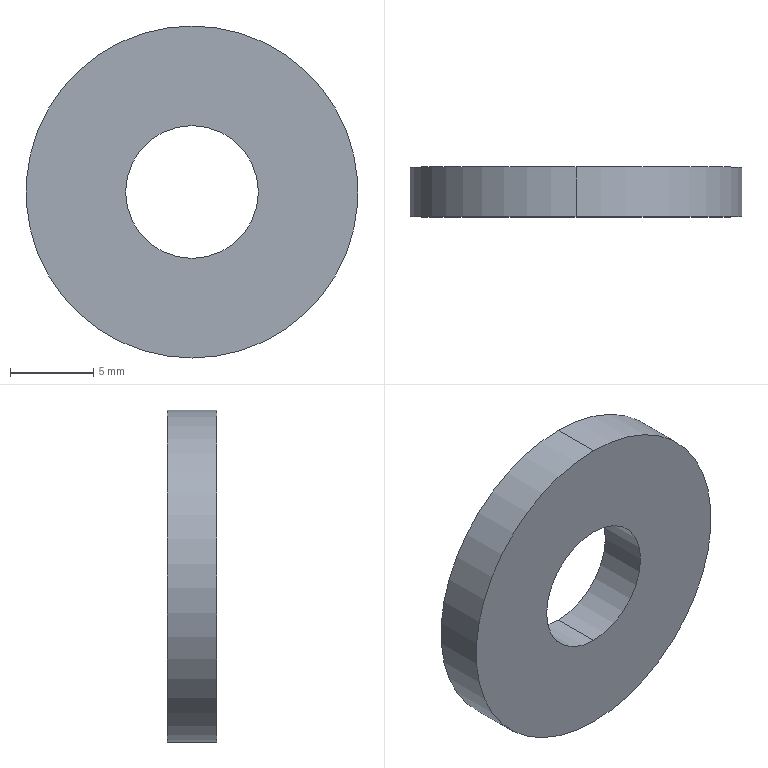Part | STEP file | Cuon T phu H01_8 | 1 solid | 6 faces | box 20 x 3 x 20 mm | volume 791.681 mm3 | cylinder 4 | plane 2 | commonest cylinder face diameters 8 x2 20 x2
STEP:
#1=CARTESIAN_POINT('',(0.,0.,0.));
#2=DIRECTION('',(0.,0.,1.));
#3=DIRECTION('',(1.,0.,0.));
#4=AXIS2_PLACEMENT_3D('',#1,#2,#3);
#5=CARTESIAN_POINT('',(0.,3.,-4.));
#6=VERTEX_POINT('',#5);
#7=CARTESIAN_POINT('',(0.,0.,-4.));
#8=VERTEX_POINT('',#7);
#9=CARTESIAN_POINT('',(0.,3.,-4.));
#10=DIRECTION('',(0.,-1.,0.));
#11=VECTOR('',#10,1.);
#12=LINE('',#9,#11);
#13=CARTESIAN_POINT('',(0.,3.,0.));
#14=DIRECTION('',(0.,-1.,0.));
#15=DIRECTION('',(0.,0.,-1.));
#16=AXIS2_PLACEMENT_3D('',#13,#14,#15);
#17=CYLINDRICAL_SURFACE('',#16,4.);
#18=CARTESIAN_POINT('',(6.283,0.));
#19=DIRECTION('',(0.,1.));
#20=VECTOR('',#19,1.);
#21=LINE('',#18,#20);
#22=(GEOMETRIC_REPRESENTATION_CONTEXT(2)PARAMETRIC_REPRESENTATION_CONTEXT()REPRESENTATION_CONTEXT('',''));
#23=DEFINITIONAL_REPRESENTATION('',(#21),#22);
#24=PCURVE('',#17,#23);
#25=CARTESIAN_POINT('',(0.,3.,0.));
#26=DIRECTION('',(0.,-1.,0.));
#27=DIRECTION('',(0.,0.,-1.));
#28=AXIS2_PLACEMENT_3D('',#25,#26,#27);
#29=CYLINDRICAL_SURFACE('',#28,4.);
#30=CARTESIAN_POINT('',(0.,0.));
#31=DIRECTION('',(0.,1.));
#32=VECTOR('',#31,1.);
#33=LINE('',#30,#32);
#34=(GEOMETRIC_REPRESENTATION_CONTEXT(2)PARAMETRIC_REPRESENTATION_CONTEXT()REPRESENTATION_CONTEXT('',''));
#35=DEFINITIONAL_REPRESENTATION('',(#33),#34);
#36=PCURVE('',#29,#35);
#37=SURFACE_CURVE('',#12,(#24,#36),.PCURVE_S1.);
#38=EDGE_CURVE('',#6,#8,#37,.T.);
#39=ORIENTED_EDGE('',*,*,#38,.T.);
#40=CARTESIAN_POINT('',(0.,0.,4.));
#41=VERTEX_POINT('',#40);
#42=CARTESIAN_POINT('',(0.,0.,0.));
#43=DIRECTION('',(0.,1.,0.));
#44=DIRECTION('',(0.,0.,1.));
#45=AXIS2_PLACEMENT_3D('',#42,#43,#44);
#46=CIRCLE('',#45,4.);
#47=CARTESIAN_POINT('',(9.425,3.));
#48=DIRECTION('',(-1.,0.));
#49=VECTOR('',#48,1.);
#50=LINE('',#47,#49);
#51=(GEOMETRIC_REPRESENTATION_CONTEXT(2)PARAMETRIC_REPRESENTATION_CONTEXT()REPRESENTATION_CONTEXT('',''));
#52=DEFINITIONAL_REPRESENTATION('',(#50),#51);
#53=PCURVE('',#17,#52);
#54=CARTESIAN_POINT('',(0.,0.,0.));
#55=DIRECTION('',(0.,1.,0.));
#56=DIRECTION('',(0.,0.,1.));
#57=AXIS2_PLACEMENT_3D('',#54,#55,#56);
#58=PLANE('',#57);
#59=CARTESIAN_POINT('',(0.,0.));
#60=DIRECTION('',(1.,0.));
#61=AXIS2_PLACEMENT_2D('',#59,#60);
#62=CIRCLE('',#61,4.);
#63=(GEOMETRIC_REPRESENTATION_CONTEXT(2)PARAMETRIC_REPRESENTATION_CONTEXT()REPRESENTATION_CONTEXT('',''));
#64=DEFINITIONAL_REPRESENTATION('',(#62),#63);
#65=PCURVE('',#58,#64);
#66=SURFACE_CURVE('',#46,(#53,#65),.PCURVE_S1.);
#67=EDGE_CURVE('',#8,#41,#66,.T.);
#68=ORIENTED_EDGE('',*,*,#67,.T.);
#69=CARTESIAN_POINT('',(0.,3.,4.));
#70=VERTEX_POINT('',#69);
#71=CARTESIAN_POINT('',(0.,3.,4.));
#72=DIRECTION('',(0.,-1.,0.));
#73=VECTOR('',#72,1.);
#74=LINE('',#71,#73);
#75=CARTESIAN_POINT('',(3.142,0.));
#76=DIRECTION('',(0.,1.));
#77=VECTOR('',#76,1.);
#78=LINE('',#75,#77);
#79=(GEOMETRIC_REPRESENTATION_CONTEXT(2)PARAMETRIC_REPRESENTATION_CONTEXT()REPRESENTATION_CONTEXT('',''));
#80=DEFINITIONAL_REPRESENTATION('',(#78),#79);
#81=PCURVE('',#17,#80);
#82=CARTESIAN_POINT('',(3.142,0.));
#83=DIRECTION('',(0.,1.));
#84=VECTOR('',#83,1.);
#85=LINE('',#82,#84);
#86=(GEOMETRIC_REPRESENTATION_CONTEXT(2)PARAMETRIC_REPRESENTATION_CONTEXT()REPRESENTATION_CONTEXT('',''));
#87=DEFINITIONAL_REPRESENTATION('',(#85),#86);
#88=PCURVE('',#29,#87);
#89=SURFACE_CURVE('',#74,(#81,#88),.PCURVE_S1.);
#90=EDGE_CURVE('',#70,#41,#89,.T.);
#91=ORIENTED_EDGE('',*,*,#90,.F.);
#92=CARTESIAN_POINT('',(0.,3.,0.));
#93=DIRECTION('',(0.,1.,0.));
#94=DIRECTION('',(0.,0.,1.));
#95=AXIS2_PLACEMENT_3D('',#92,#93,#94);
#96=CIRCLE('',#95,4.);
#97=CARTESIAN_POINT('',(9.425,0.));
#98=DIRECTION('',(-1.,0.));
#99=VECTOR('',#98,1.);
#100=LINE('',#97,#99);
#101=(GEOMETRIC_REPRESENTATION_CONTEXT(2)PARAMETRIC_REPRESENTATION_CONTEXT()REPRESENTATION_CONTEXT('',''));
#102=DEFINITIONAL_REPRESENTATION('',(#100),#101);
#103=PCURVE('',#17,#102);
#104=CARTESIAN_POINT('',(0.,3.,0.));
#105=DIRECTION('',(0.,1.,0.));
#106=DIRECTION('',(0.,0.,1.));
#107=AXIS2_PLACEMENT_3D('',#104,#105,#106);
#108=PLANE('',#107);
#109=CARTESIAN_POINT('',(0.,0.));
#110=DIRECTION('',(1.,0.));
#111=AXIS2_PLACEMENT_2D('',#109,#110);
#112=CIRCLE('',#111,4.);
#113=(GEOMETRIC_REPRESENTATION_CONTEXT(2)PARAMETRIC_REPRESENTATION_CONTEXT()REPRESENTATION_CONTEXT('',''));
#114=DEFINITIONAL_REPRESENTATION('',(#112),#113);
#115=PCURVE('',#108,#114);
#116=SURFACE_CURVE('',#96,(#103,#115),.PCURVE_S1.);
#117=EDGE_CURVE('',#6,#70,#116,.T.);
#118=ORIENTED_EDGE('',*,*,#117,.F.);
#119=EDGE_LOOP('',(#39,#68,#91,#118));
#120=FACE_BOUND('',#119,.F.);
#121=ADVANCED_FACE('',(#120),#17,.F.);
#122=CARTESIAN_POINT('',(0.,3.,10.));
#123=VERTEX_POINT('',#122);
#124=CARTESIAN_POINT('',(0.,3.,-10.));
#125=VERTEX_POINT('',#124);
#126=CARTESIAN_POINT('',(0.,3.,0.));
#127=DIRECTION('',(0.,1.,0.));
#128=DIRECTION('',(0.,0.,1.));
#129=AXIS2_PLACEMENT_3D('',#126,#127,#128);
#130=CIRCLE('',#129,10.);
#131=CARTESIAN_POINT('',(0.,3.,0.));
#132=DIRECTION('',(0.,-1.,0.));
#133=DIRECTION('',(0.,0.,-1.));
#134=AXIS2_PLACEMENT_3D('',#131,#132,#133);
#135=CYLINDRICAL_SURFACE('',#134,10.);
#136=CARTESIAN_POINT('',(3.142,0.));
#137=DIRECTION('',(-1.,0.));
#138=VECTOR('',#137,1.);
#139=LINE('',#136,#138);
#140=(GEOMETRIC_REPRESENTATION_CONTEXT(2)PARAMETRIC_REPRESENTATION_CONTEXT()REPRESENTATION_CONTEXT('',''));
#141=DEFINITIONAL_REPRESENTATION('',(#139),#140);
#142=PCURVE('',#135,#141);
#143=CARTESIAN_POINT('',(0.,0.));
#144=DIRECTION('',(1.,0.));
#145=AXIS2_PLACEMENT_2D('',#143,#144);
#146=CIRCLE('',#145,10.);
#147=(GEOMETRIC_REPRESENTATION_CONTEXT(2)PARAMETRIC_REPRESENTATION_CONTEXT()REPRESENTATION_CONTEXT('',''));
#148=DEFINITIONAL_REPRESENTATION('',(#146),#147);
#149=PCURVE('',#108,#148);
#150=SURFACE_CURVE('',#130,(#142,#149),.PCURVE_S1.);
#151=EDGE_CURVE('',#123,#125,#150,.T.);
#152=ORIENTED_EDGE('',*,*,#151,.F.);
#153=CARTESIAN_POINT('',(0.,0.,10.));
#154=VERTEX_POINT('',#153);
#155=CARTESIAN_POINT('',(0.,3.,10.));
#156=DIRECTION('',(0.,-1.,0.));
#157=VECTOR('',#156,1.);
#158=LINE('',#155,#157);
#159=CARTESIAN_POINT('',(3.142,0.));
#160=DIRECTION('',(0.,1.));
#161=VECTOR('',#160,1.);
#162=LINE('',#159,#161);
#163=(GEOMETRIC_REPRESENTATION_CONTEXT(2)PARAMETRIC_REPRESENTATION_CONTEXT()REPRESENTATION_CONTEXT('',''));
#164=DEFINITIONAL_REPRESENTATION('',(#162),#163);
#165=PCURVE('',#135,#164);
#166=CARTESIAN_POINT('',(0.,3.,0.));
#167=DIRECTION('',(0.,-1.,0.));
#168=DIRECTION('',(0.,0.,-1.));
#169=AXIS2_PLACEMENT_3D('',#166,#167,#168);
#170=CYLINDRICAL_SURFACE('',#169,10.);
#171=CARTESIAN_POINT('',(3.142,0.));
#172=DIRECTION('',(0.,1.));
#173=VECTOR('',#172,1.);
#174=LINE('',#171,#173);
#175=(GEOMETRIC_REPRESENTATION_CONTEXT(2)PARAMETRIC_REPRESENTATION_CONTEXT()REPRESENTATION_CONTEXT('',''));
#176=DEFINITIONAL_REPRESENTATION('',(#174),#175);
#177=PCURVE('',#170,#176);
#178=SURFACE_CURVE('',#158,(#165,#177),.PCURVE_S1.);
#179=EDGE_CURVE('',#123,#154,#178,.T.);
#180=ORIENTED_EDGE('',*,*,#179,.T.);
#181=CARTESIAN_POINT('',(0.,0.,-10.));
#182=VERTEX_POINT('',#181);
#183=CARTESIAN_POINT('',(0.,0.,0.));
#184=DIRECTION('',(0.,1.,0.));
#185=DIRECTION('',(0.,0.,1.));
#186=AXIS2_PLACEMENT_3D('',#183,#184,#185);
#187=CIRCLE('',#186,10.);
#188=CARTESIAN_POINT('',(3.142,3.));
#189=DIRECTION('',(-1.,0.));
#190=VECTOR('',#189,1.);
#191=LINE('',#188,#190);
#192=(GEOMETRIC_REPRESENTATION_CONTEXT(2)PARAMETRIC_REPRESENTATION_CONTEXT()REPRESENTATION_CONTEXT('',''));
#193=DEFINITIONAL_REPRESENTATION('',(#191),#192);
#194=PCURVE('',#135,#193);
#195=CARTESIAN_POINT('',(0.,0.));
#196=DIRECTION('',(1.,0.));
#197=AXIS2_PLACEMENT_2D('',#195,#196);
#198=CIRCLE('',#197,10.);
#199=(GEOMETRIC_REPRESENTATION_CONTEXT(2)PARAMETRIC_REPRESENTATION_CONTEXT()REPRESENTATION_CONTEXT('',''));
#200=DEFINITIONAL_REPRESENTATION('',(#198),#199);
#201=PCURVE('',#58,#200);
#202=SURFACE_CURVE('',#187,(#194,#201),.PCURVE_S1.);
#203=EDGE_CURVE('',#154,#182,#202,.T.);
#204=ORIENTED_EDGE('',*,*,#203,.T.);
#205=CARTESIAN_POINT('',(0.,3.,-10.));
#206=DIRECTION('',(0.,-1.,0.));
#207=VECTOR('',#206,1.);
#208=LINE('',#205,#207);
#209=CARTESIAN_POINT('',(0.,0.));
#210=DIRECTION('',(0.,1.));
#211=VECTOR('',#210,1.);
#212=LINE('',#209,#211);
#213=(GEOMETRIC_REPRESENTATION_CONTEXT(2)PARAMETRIC_REPRESENTATION_CONTEXT()REPRESENTATION_CONTEXT('',''));
#214=DEFINITIONAL_REPRESENTATION('',(#212),#213);
#215=PCURVE('',#135,#214);
#216=CARTESIAN_POINT('',(6.283,0.));
#217=DIRECTION('',(0.,1.));
#218=VECTOR('',#217,1.);
#219=LINE('',#216,#218);
#220=(GEOMETRIC_REPRESENTATION_CONTEXT(2)PARAMETRIC_REPRESENTATION_CONTEXT()REPRESENTATION_CONTEXT('',''));
#221=DEFINITIONAL_REPRESENTATION('',(#219),#220);
#222=PCURVE('',#170,#221);
#223=SURFACE_CURVE('',#208,(#215,#222),.PCURVE_S1.);
#224=EDGE_CURVE('',#125,#182,#223,.T.);
#225=ORIENTED_EDGE('',*,*,#224,.F.);
#226=EDGE_LOOP('',(#152,#180,#204,#225));
#227=FACE_BOUND('',#226,.T.);
#228=ADVANCED_FACE('',(#227),#135,.T.);
#229=CARTESIAN_POINT('',(0.,3.,0.));
#230=DIRECTION('',(0.,1.,0.));
#231=DIRECTION('',(0.,0.,1.));
#232=AXIS2_PLACEMENT_3D('',#229,#230,#231);
#233=CIRCLE('',#232,10.);
#234=CARTESIAN_POINT('',(0.,0.));
#235=DIRECTION('',(1.,0.));
#236=AXIS2_PLACEMENT_2D('',#234,#235);
#237=CIRCLE('',#236,10.);
#238=(GEOMETRIC_REPRESENTATION_CONTEXT(2)PARAMETRIC_REPRESENTATION_CONTEXT()REPRESENTATION_CONTEXT('',''));
#239=DEFINITIONAL_REPRESENTATION('',(#237),#238);
#240=PCURVE('',#108,#239);
#241=CARTESIAN_POINT('',(9.425,0.));
#242=DIRECTION('',(-1.,0.));
#243=VECTOR('',#242,1.);
#244=LINE('',#241,#243);
#245=(GEOMETRIC_REPRESENTATION_CONTEXT(2)PARAMETRIC_REPRESENTATION_CONTEXT()REPRESENTATION_CONTEXT('',''));
#246=DEFINITIONAL_REPRESENTATION('',(#244),#245);
#247=PCURVE('',#170,#246);
#248=SURFACE_CURVE('',#233,(#240,#247),.PCURVE_S1.);
#249=EDGE_CURVE('',#125,#123,#248,.T.);
#250=ORIENTED_EDGE('',*,*,#249,.T.);
#251=ORIENTED_EDGE('',*,*,#151,.T.);
#252=EDGE_LOOP('',(#250,#251));
#253=FACE_BOUND('',#252,.T.);
#254=ORIENTED_EDGE('',*,*,#117,.F.);
#255=CARTESIAN_POINT('',(0.,3.,0.));
#256=DIRECTION('',(0.,1.,0.));
#257=DIRECTION('',(0.,0.,1.));
#258=AXIS2_PLACEMENT_3D('',#255,#256,#257);
#259=CIRCLE('',#258,4.);
#260=CARTESIAN_POINT('',(0.,0.));
#261=DIRECTION('',(1.,0.));
#262=AXIS2_PLACEMENT_2D('',#260,#261);
#263=CIRCLE('',#262,4.);
#264=(GEOMETRIC_REPRESENTATION_CONTEXT(2)PARAMETRIC_REPRESENTATION_CONTEXT()REPRESENTATION_CONTEXT('',''));
#265=DEFINITIONAL_REPRESENTATION('',(#263),#264);
#266=PCURVE('',#108,#265);
#267=CARTESIAN_POINT('',(3.142,0.));
#268=DIRECTION('',(-1.,0.));
#269=VECTOR('',#268,1.);
#270=LINE('',#267,#269);
#271=(GEOMETRIC_REPRESENTATION_CONTEXT(2)PARAMETRIC_REPRESENTATION_CONTEXT()REPRESENTATION_CONTEXT('',''));
#272=DEFINITIONAL_REPRESENTATION('',(#270),#271);
#273=PCURVE('',#29,#272);
#274=SURFACE_CURVE('',#259,(#266,#273),.PCURVE_S1.);
#275=EDGE_CURVE('',#70,#6,#274,.T.);
#276=ORIENTED_EDGE('',*,*,#275,.F.);
#277=EDGE_LOOP('',(#254,#276));
#278=FACE_BOUND('',#277,.T.);
#279=ADVANCED_FACE('',(#253,#278),#108,.T.);
#280=CARTESIAN_POINT('',(0.,0.,0.));
#281=DIRECTION('',(0.,1.,0.));
#282=DIRECTION('',(0.,0.,1.));
#283=AXIS2_PLACEMENT_3D('',#280,#281,#282);
#284=CIRCLE('',#283,10.);
#285=CARTESIAN_POINT('',(0.,0.));
#286=DIRECTION('',(1.,0.));
#287=AXIS2_PLACEMENT_2D('',#285,#286);
#288=CIRCLE('',#287,10.);
#289=(GEOMETRIC_REPRESENTATION_CONTEXT(2)PARAMETRIC_REPRESENTATION_CONTEXT()REPRESENTATION_CONTEXT('',''));
#290=DEFINITIONAL_REPRESENTATION('',(#288),#289);
#291=PCURVE('',#58,#290);
#292=CARTESIAN_POINT('',(9.425,3.));
#293=DIRECTION('',(-1.,0.));
#294=VECTOR('',#293,1.);
#295=LINE('',#292,#294);
#296=(GEOMETRIC_REPRESENTATION_CONTEXT(2)PARAMETRIC_REPRESENTATION_CONTEXT()REPRESENTATION_CONTEXT('',''));
#297=DEFINITIONAL_REPRESENTATION('',(#295),#296);
#298=PCURVE('',#170,#297);
#299=SURFACE_CURVE('',#284,(#291,#298),.PCURVE_S1.);
#300=EDGE_CURVE('',#182,#154,#299,.T.);
#301=ORIENTED_EDGE('',*,*,#300,.F.);
#302=ORIENTED_EDGE('',*,*,#203,.F.);
#303=EDGE_LOOP('',(#301,#302));
#304=FACE_BOUND('',#303,.T.);
#305=ORIENTED_EDGE('',*,*,#67,.T.);
#306=CARTESIAN_POINT('',(0.,0.,0.));
#307=DIRECTION('',(0.,1.,0.));
#308=DIRECTION('',(0.,0.,1.));
#309=AXIS2_PLACEMENT_3D('',#306,#307,#308);
#310=CIRCLE('',#309,4.);
#311=CARTESIAN_POINT('',(0.,0.));
#312=DIRECTION('',(1.,0.));
#313=AXIS2_PLACEMENT_2D('',#311,#312);
#314=CIRCLE('',#313,4.);
#315=(GEOMETRIC_REPRESENTATION_CONTEXT(2)PARAMETRIC_REPRESENTATION_CONTEXT()REPRESENTATION_CONTEXT('',''));
#316=DEFINITIONAL_REPRESENTATION('',(#314),#315);
#317=PCURVE('',#58,#316);
#318=CARTESIAN_POINT('',(3.142,3.));
#319=DIRECTION('',(-1.,0.));
#320=VECTOR('',#319,1.);
#321=LINE('',#318,#320);
#322=(GEOMETRIC_REPRESENTATION_CONTEXT(2)PARAMETRIC_REPRESENTATION_CONTEXT()REPRESENTATION_CONTEXT('',''));
#323=DEFINITIONAL_REPRESENTATION('',(#321),#322);
#324=PCURVE('',#29,#323);
#325=SURFACE_CURVE('',#310,(#317,#324),.PCURVE_S1.);
#326=EDGE_CURVE('',#41,#8,#325,.T.);
#327=ORIENTED_EDGE('',*,*,#326,.T.);
#328=EDGE_LOOP('',(#305,#327));
#329=FACE_BOUND('',#328,.T.);
#330=ADVANCED_FACE('',(#304,#329),#58,.F.);
#331=ORIENTED_EDGE('',*,*,#179,.F.);
#332=ORIENTED_EDGE('',*,*,#249,.F.);
#333=ORIENTED_EDGE('',*,*,#224,.T.);
#334=ORIENTED_EDGE('',*,*,#300,.T.);
#335=EDGE_LOOP('',(#331,#332,#333,#334));
#336=FACE_BOUND('',#335,.T.);
#337=ADVANCED_FACE('',(#336),#170,.T.);
#338=ORIENTED_EDGE('',*,*,#326,.T.);
#339=ORIENTED_EDGE('',*,*,#38,.F.);
#340=ORIENTED_EDGE('',*,*,#275,.F.);
#341=ORIENTED_EDGE('',*,*,#90,.T.);
#342=EDGE_LOOP('',(#338,#339,#340,#341));
#343=FACE_BOUND('',#342,.F.);
#344=ADVANCED_FACE('',(#343),#29,.F.);
#345=CLOSED_SHELL('',(#121,#228,#279,#330,#337,#344));
#346=MANIFOLD_SOLID_BREP('',#345);
#347=(LENGTH_UNIT()NAMED_UNIT(*)SI_UNIT(.MILLI.,.METRE.));
#348=UNCERTAINTY_MEASURE_WITH_UNIT(LENGTH_MEASURE(0.0000001),#347,'','');
#349=(NAMED_UNIT(*)PLANE_ANGLE_UNIT()SI_UNIT($,.RADIAN.));
#350=(NAMED_UNIT(*)SI_UNIT($,.STERADIAN.)SOLID_ANGLE_UNIT());
#351=(GEOMETRIC_REPRESENTATION_CONTEXT(3)GLOBAL_UNCERTAINTY_ASSIGNED_CONTEXT((#348))GLOBAL_UNIT_ASSIGNED_CONTEXT((#347,#349,#350))REPRESENTATION_CONTEXT('',''));
#352=ADVANCED_BREP_SHAPE_REPRESENTATION('',(#4,#346),#351);